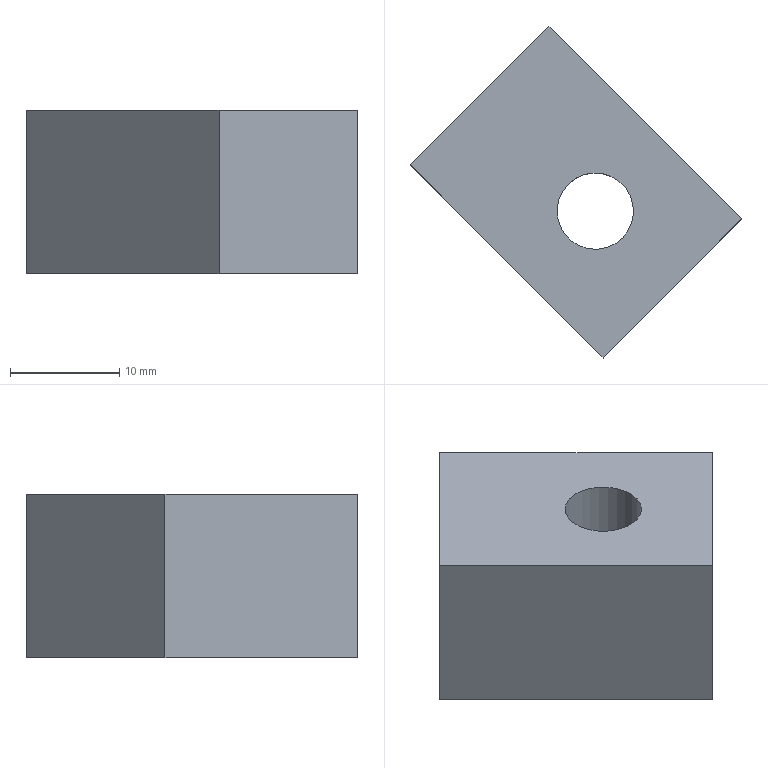Part | STEP file | PN_0010_id1734_x_t | 1 solid | 9 faces | box 30.406 x 30.406 x 15 mm | volume 5664 mm3 | plane 7 | cylinder 2 | commonest cylinder face diameters 7 x1 11 x1
STEP:
#1=CARTESIAN_POINT('',(-258.929,-172.299,105.));
#2=VERTEX_POINT('',#1);
#3=CARTESIAN_POINT('',(-241.251,-189.977,105.));
#4=VERTEX_POINT('',#3);
#5=CARTESIAN_POINT('',(-258.929,-172.299,105.));
#6=DIRECTION('',(0.7071,-0.7071,0.));
#7=VECTOR('',#6,1.);
#8=LINE('',#5,#7);
#9=EDGE_CURVE('',#2,#4,#8,.T.);
#10=ORIENTED_EDGE('',*,*,#9,.F.);
#11=CARTESIAN_POINT('',(-258.929,-172.299,90.));
#12=VERTEX_POINT('',#11);
#13=CARTESIAN_POINT('',(-258.929,-172.299,105.));
#14=DIRECTION('',(0.,0.,-1.));
#15=VECTOR('',#14,1.);
#16=LINE('',#13,#15);
#17=EDGE_CURVE('',#2,#12,#16,.T.);
#18=ORIENTED_EDGE('',*,*,#17,.T.);
#19=CARTESIAN_POINT('',(-241.251,-189.977,90.));
#20=VERTEX_POINT('',#19);
#21=CARTESIAN_POINT('',(-258.929,-172.299,90.));
#22=DIRECTION('',(0.7071,-0.7071,0.));
#23=VECTOR('',#22,1.);
#24=LINE('',#21,#23);
#25=EDGE_CURVE('',#12,#20,#24,.T.);
#26=ORIENTED_EDGE('',*,*,#25,.T.);
#27=CARTESIAN_POINT('',(-241.251,-189.977,105.));
#28=DIRECTION('',(0.,0.,-1.));
#29=VECTOR('',#28,1.);
#30=LINE('',#27,#29);
#31=EDGE_CURVE('',#4,#20,#30,.T.);
#32=ORIENTED_EDGE('',*,*,#31,.F.);
#33=EDGE_LOOP('',(#10,#18,#26,#32));
#34=FACE_OUTER_BOUND('',#33,.T.);
#35=CARTESIAN_POINT('',(-258.929,-172.299,105.));
#36=DIRECTION('',(-0.7071,-0.7071,0.));
#37=DIRECTION('',(0.,0.,-1.));
#38=AXIS2_PLACEMENT_3D('',#35,#36,#37);
#39=PLANE('',#38);
#40=ADVANCED_FACE('',(#34),#39,.T.);
#41=CARTESIAN_POINT('',(-245.847,-172.653,90.));
#42=VERTEX_POINT('',#41);
#43=CARTESIAN_POINT('',(-241.958,-176.542,90.));
#44=DIRECTION('',(0.,0.,1.));
#45=DIRECTION('',(-0.7071,0.7071,0.));
#46=AXIS2_PLACEMENT_3D('',#43,#44,#45);
#47=CIRCLE('',#46,5.5);
#48=EDGE_CURVE('',#42,#42,#47,.T.);
#49=ORIENTED_EDGE('',*,*,#48,.T.);
#50=EDGE_LOOP('',(#49));
#51=FACE_BOUND('',#50,.T.);
#52=ORIENTED_EDGE('',*,*,#25,.F.);
#53=CARTESIAN_POINT('',(-246.201,-159.571,90.));
#54=VERTEX_POINT('',#53);
#55=CARTESIAN_POINT('',(-252.565,-165.935,90.));
#56=DIRECTION('',(0.7071,0.7071,0.));
#57=VECTOR('',#56,1.);
#58=LINE('',#55,#57);
#59=EDGE_CURVE('',#12,#54,#58,.T.);
#60=ORIENTED_EDGE('',*,*,#59,.T.);
#61=CARTESIAN_POINT('',(-228.523,-177.249,90.));
#62=VERTEX_POINT('',#61);
#63=CARTESIAN_POINT('',(-246.201,-159.571,90.));
#64=DIRECTION('',(0.7071,-0.7071,0.));
#65=VECTOR('',#64,1.);
#66=LINE('',#63,#65);
#67=EDGE_CURVE('',#54,#62,#66,.T.);
#68=ORIENTED_EDGE('',*,*,#67,.T.);
#69=CARTESIAN_POINT('',(-234.887,-183.613,90.));
#70=DIRECTION('',(0.7071,0.7071,0.));
#71=VECTOR('',#70,1.);
#72=LINE('',#69,#71);
#73=EDGE_CURVE('',#20,#62,#72,.T.);
#74=ORIENTED_EDGE('',*,*,#73,.F.);
#75=EDGE_LOOP('',(#52,#60,#68,#74));
#76=FACE_BOUND('',#75,.T.);
#77=CARTESIAN_POINT('',(-252.565,-165.935,90.));
#78=DIRECTION('',(0.,0.,-1.));
#79=DIRECTION('',(0.7071,0.7071,0.));
#80=AXIS2_PLACEMENT_3D('',#77,#78,#79);
#81=PLANE('',#80);
#82=ADVANCED_FACE('',(#51,#76),#81,.T.);
#83=ORIENTED_EDGE('',*,*,#67,.F.);
#84=CARTESIAN_POINT('',(-246.201,-159.571,105.));
#85=VERTEX_POINT('',#84);
#86=CARTESIAN_POINT('',(-246.201,-159.571,105.));
#87=DIRECTION('',(0.,0.,-1.));
#88=VECTOR('',#87,1.);
#89=LINE('',#86,#88);
#90=EDGE_CURVE('',#85,#54,#89,.T.);
#91=ORIENTED_EDGE('',*,*,#90,.F.);
#92=CARTESIAN_POINT('',(-228.523,-177.249,105.));
#93=VERTEX_POINT('',#92);
#94=CARTESIAN_POINT('',(-246.201,-159.571,105.));
#95=DIRECTION('',(0.7071,-0.7071,0.));
#96=VECTOR('',#95,1.);
#97=LINE('',#94,#96);
#98=EDGE_CURVE('',#85,#93,#97,.T.);
#99=ORIENTED_EDGE('',*,*,#98,.T.);
#100=CARTESIAN_POINT('',(-228.523,-177.249,105.));
#101=DIRECTION('',(0.,0.,-1.));
#102=VECTOR('',#101,1.);
#103=LINE('',#100,#102);
#104=EDGE_CURVE('',#93,#62,#103,.T.);
#105=ORIENTED_EDGE('',*,*,#104,.T.);
#106=EDGE_LOOP('',(#83,#91,#99,#105));
#107=FACE_OUTER_BOUND('',#106,.T.);
#108=CARTESIAN_POINT('',(-246.201,-159.571,105.));
#109=DIRECTION('',(-0.7071,-0.7071,0.));
#110=DIRECTION('',(0.,0.,-1.));
#111=AXIS2_PLACEMENT_3D('',#108,#109,#110);
#112=PLANE('',#111);
#113=ADVANCED_FACE('',(#107),#112,.F.);
#114=CARTESIAN_POINT('',(-244.433,-174.067,105.));
#115=VERTEX_POINT('',#114);
#116=CARTESIAN_POINT('',(-241.958,-176.542,105.));
#117=DIRECTION('',(0.,0.,-1.));
#118=DIRECTION('',(-0.7071,0.7071,0.));
#119=AXIS2_PLACEMENT_3D('',#116,#117,#118);
#120=CIRCLE('',#119,3.5);
#121=EDGE_CURVE('',#115,#115,#120,.T.);
#122=ORIENTED_EDGE('',*,*,#121,.T.);
#123=EDGE_LOOP('',(#122));
#124=FACE_BOUND('',#123,.T.);
#125=CARTESIAN_POINT('',(-252.565,-165.935,105.));
#126=DIRECTION('',(0.7071,0.7071,0.));
#127=VECTOR('',#126,1.);
#128=LINE('',#125,#127);
#129=EDGE_CURVE('',#2,#85,#128,.T.);
#130=ORIENTED_EDGE('',*,*,#129,.F.);
#131=ORIENTED_EDGE('',*,*,#9,.T.);
#132=CARTESIAN_POINT('',(-234.887,-183.613,105.));
#133=DIRECTION('',(0.7071,0.7071,0.));
#134=VECTOR('',#133,1.);
#135=LINE('',#132,#134);
#136=EDGE_CURVE('',#4,#93,#135,.T.);
#137=ORIENTED_EDGE('',*,*,#136,.T.);
#138=ORIENTED_EDGE('',*,*,#98,.F.);
#139=EDGE_LOOP('',(#130,#131,#137,#138));
#140=FACE_BOUND('',#139,.T.);
#141=CARTESIAN_POINT('',(-252.565,-165.935,105.));
#142=DIRECTION('',(0.,0.,1.));
#143=DIRECTION('',(-0.7071,-0.7071,0.));
#144=AXIS2_PLACEMENT_3D('',#141,#142,#143);
#145=PLANE('',#144);
#146=ADVANCED_FACE('',(#124,#140),#145,.T.);
#147=ORIENTED_EDGE('',*,*,#104,.F.);
#148=ORIENTED_EDGE('',*,*,#136,.F.);
#149=ORIENTED_EDGE('',*,*,#31,.T.);
#150=ORIENTED_EDGE('',*,*,#73,.T.);
#151=EDGE_LOOP('',(#147,#148,#149,#150));
#152=FACE_OUTER_BOUND('',#151,.T.);
#153=CARTESIAN_POINT('',(-234.887,-183.613,105.));
#154=DIRECTION('',(0.7071,-0.7071,0.));
#155=DIRECTION('',(-0.7071,-0.7071,0.));
#156=AXIS2_PLACEMENT_3D('',#153,#154,#155);
#157=PLANE('',#156);
#158=ADVANCED_FACE('',(#152),#157,.T.);
#159=ORIENTED_EDGE('',*,*,#90,.T.);
#160=ORIENTED_EDGE('',*,*,#59,.F.);
#161=ORIENTED_EDGE('',*,*,#17,.F.);
#162=ORIENTED_EDGE('',*,*,#129,.T.);
#163=EDGE_LOOP('',(#159,#160,#161,#162));
#164=FACE_OUTER_BOUND('',#163,.T.);
#165=CARTESIAN_POINT('',(-252.565,-165.935,105.));
#166=DIRECTION('',(0.7071,-0.7071,0.));
#167=DIRECTION('',(-0.7071,-0.7071,0.));
#168=AXIS2_PLACEMENT_3D('',#165,#166,#167);
#169=PLANE('',#168);
#170=ADVANCED_FACE('',(#164),#169,.F.);
#171=CARTESIAN_POINT('',(-239.483,-179.017,99.));
#172=VERTEX_POINT('',#171);
#173=CARTESIAN_POINT('',(-241.958,-176.542,99.));
#174=DIRECTION('',(0.,0.,1.));
#175=DIRECTION('',(0.7071,-0.7071,0.));
#176=AXIS2_PLACEMENT_3D('',#173,#174,#175);
#177=CIRCLE('',#176,3.5);
#178=EDGE_CURVE('',#172,#172,#177,.T.);
#179=ORIENTED_EDGE('',*,*,#178,.F.);
#180=EDGE_LOOP('',(#179));
#181=FACE_BOUND('',#180,.T.);
#182=ORIENTED_EDGE('',*,*,#121,.F.);
#183=EDGE_LOOP('',(#182));
#184=FACE_BOUND('',#183,.T.);
#185=CARTESIAN_POINT('',(-241.958,-176.542,105.));
#186=DIRECTION('',(0.,0.,-1.));
#187=DIRECTION('',(-0.7071,0.7071,0.));
#188=AXIS2_PLACEMENT_3D('',#185,#186,#187);
#189=CYLINDRICAL_SURFACE('',#188,3.5);
#190=ADVANCED_FACE('',(#181,#184),#189,.F.);
#191=ORIENTED_EDGE('',*,*,#178,.T.);
#192=EDGE_LOOP('',(#191));
#193=FACE_BOUND('',#192,.T.);
#194=CARTESIAN_POINT('',(-245.847,-172.653,99.));
#195=VERTEX_POINT('',#194);
#196=CARTESIAN_POINT('',(-241.958,-176.542,99.));
#197=DIRECTION('',(0.,0.,1.));
#198=DIRECTION('',(-0.7071,0.7071,0.));
#199=AXIS2_PLACEMENT_3D('',#196,#197,#198);
#200=CIRCLE('',#199,5.5);
#201=EDGE_CURVE('',#195,#195,#200,.T.);
#202=ORIENTED_EDGE('',*,*,#201,.F.);
#203=EDGE_LOOP('',(#202));
#204=FACE_BOUND('',#203,.T.);
#205=CARTESIAN_POINT('',(-241.958,-176.542,99.));
#206=DIRECTION('',(0.,0.,1.));
#207=DIRECTION('',(0.7071,-0.7071,0.));
#208=AXIS2_PLACEMENT_3D('',#205,#206,#207);
#209=PLANE('',#208);
#210=ADVANCED_FACE('',(#193,#204),#209,.F.);
#211=ORIENTED_EDGE('',*,*,#48,.F.);
#212=EDGE_LOOP('',(#211));
#213=FACE_BOUND('',#212,.T.);
#214=ORIENTED_EDGE('',*,*,#201,.T.);
#215=EDGE_LOOP('',(#214));
#216=FACE_BOUND('',#215,.T.);
#217=CARTESIAN_POINT('',(-241.958,-176.542,99.));
#218=DIRECTION('',(0.,0.,-1.));
#219=DIRECTION('',(-0.7071,0.7071,0.));
#220=AXIS2_PLACEMENT_3D('',#217,#218,#219);
#221=CYLINDRICAL_SURFACE('',#220,5.5);
#222=ADVANCED_FACE('',(#213,#216),#221,.F.);
#223=CLOSED_SHELL('',(#40,#82,#113,#146,#158,#170,#190,#210,#222));
#224=MANIFOLD_SOLID_BREP('',#223);
#225=(LENGTH_UNIT()NAMED_UNIT(*)SI_UNIT(.MILLI.,.METRE.));
#226=UNCERTAINTY_MEASURE_WITH_UNIT(LENGTH_MEASURE(0.00002),#225,'','');
#227=(NAMED_UNIT(*)PLANE_ANGLE_UNIT()SI_UNIT($,.RADIAN.));
#228=PLANE_ANGLE_MEASURE_WITH_UNIT(PLANE_ANGLE_MEASURE(0.01745),#227);
#229=DIMENSIONAL_EXPONENTS(0.,0.,0.,0.,0.,0.,0.);
#230=(CONVERSION_BASED_UNIT('DEGREE',#228)NAMED_UNIT(#229)PLANE_ANGLE_UNIT());
#231=(NAMED_UNIT(*)SI_UNIT($,.STERADIAN.)SOLID_ANGLE_UNIT());
#232=(GEOMETRIC_REPRESENTATION_CONTEXT(3)GLOBAL_UNCERTAINTY_ASSIGNED_CONTEXT((#226))GLOBAL_UNIT_ASSIGNED_CONTEXT((#225,#230,#231))REPRESENTATION_CONTEXT('',''));
#233=ADVANCED_BREP_SHAPE_REPRESENTATION('',(#224),#232);